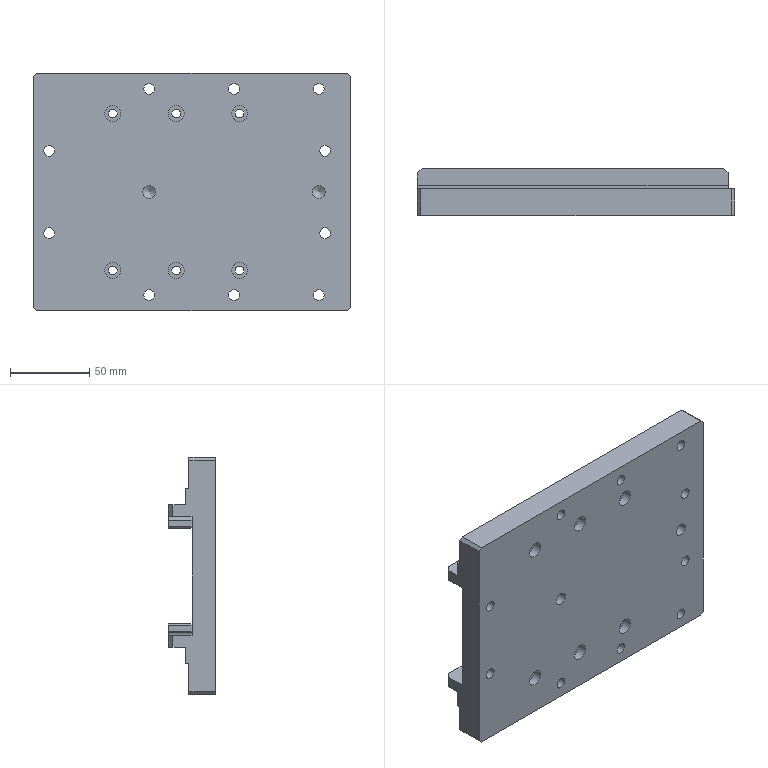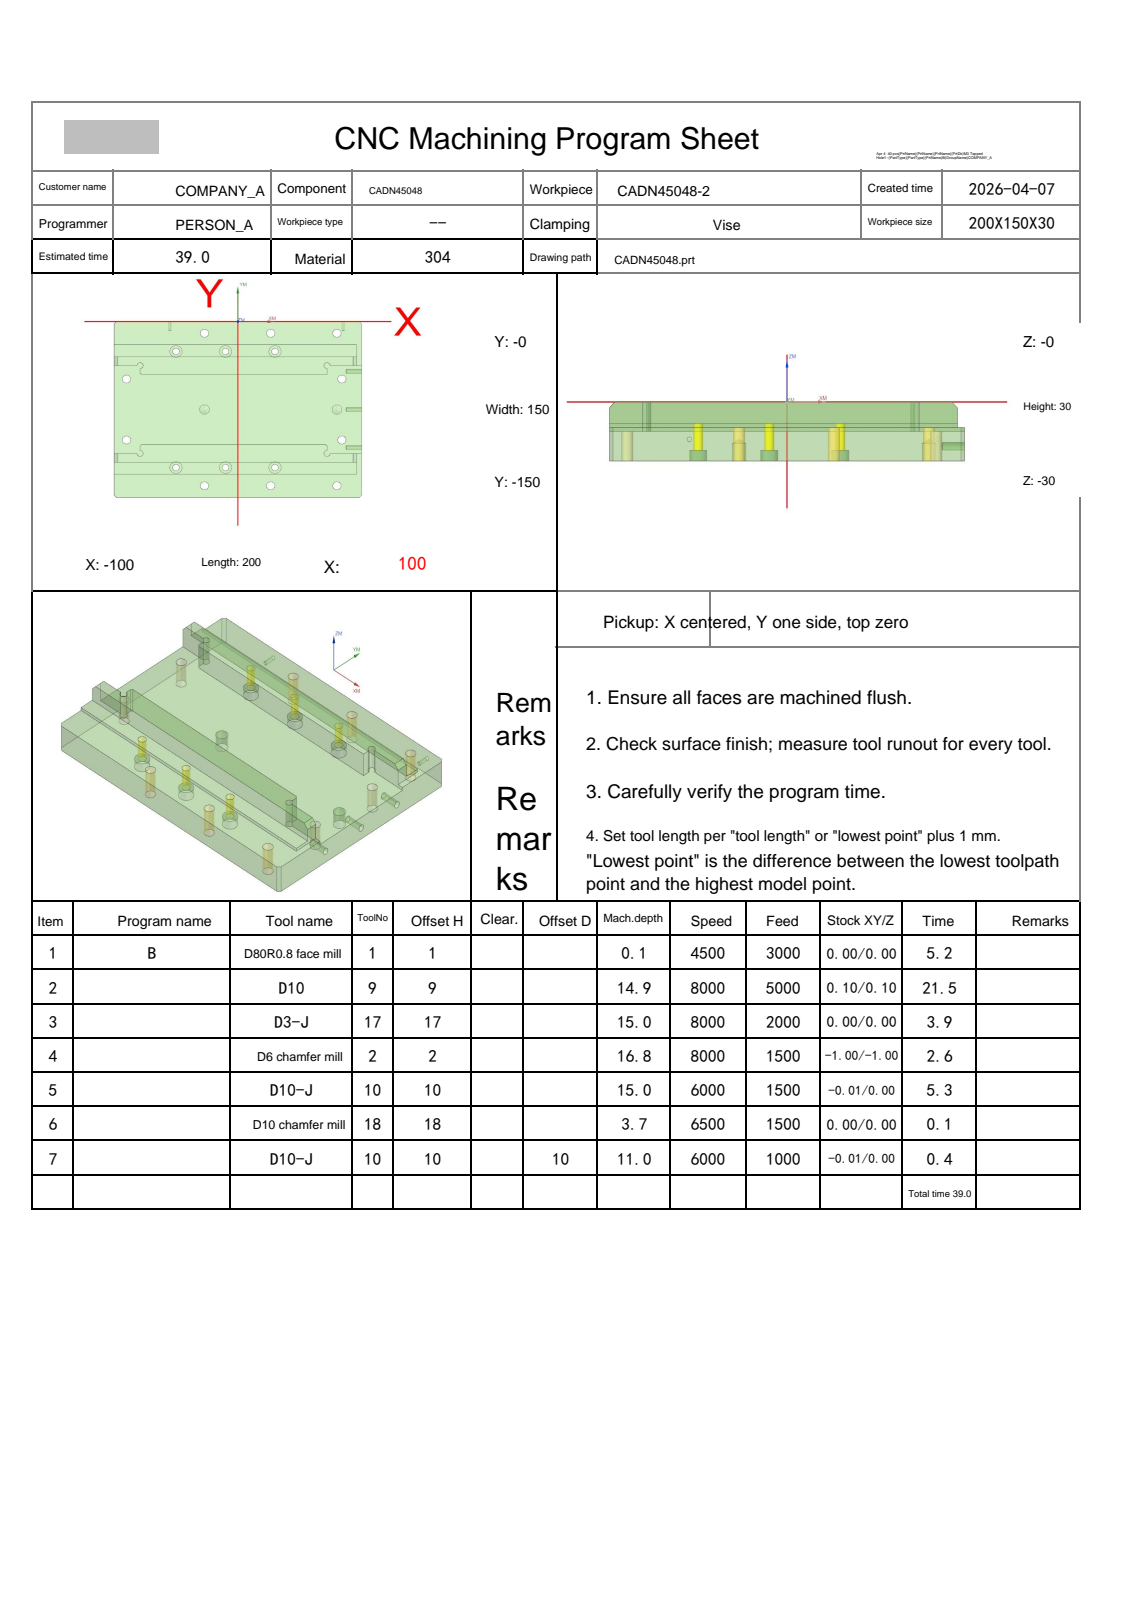NC program | NX | posted by the shop | part box 200 x 30 x 150 mm
Lines 18128 to 19220 of 19220:
N4 T02 M06
(D6 chamfer mill  D=6. R=0. H=02 ce=-1.00 di=-0.80)
G00 G90 G54 X-25. Y-10. M03 S8000
G43 H02 Z20.
M08
Z-13.9
G01 Z-14.4 F600.
X-24.
G03 X-27. Y-7. I-3. J0.0
X-30. Y-10. I0.0 J-3.
X-27. Y-13. I3. J0.0
X-24. Y-10. I0.0 J3.
X-27. Y-7. I-3. J0.0
X-30. Y-10. I0.0 J-3.
G01 X-29.
Z-13.9
G00 Z20.
X28.5
Z-13.9
G01 Z-14.4
X29.5
G03 X26.5 Y-7. I-3. J0.0
X23.5 Y-10. I0.0 J-3.
X26.5 Y-13. I3. J0.0
X29.5 Y-10. I0.0 J3.
X26.5 Y-7. I-3. J0.0
X23.5 Y-10. I0.0 J-3.
G01 X24.5
Z-13.9
G00 Z20.
X82.
Z-13.9
G01 Z-14.4
X83.
G03 X80. Y-7. I-3. J0.0
X77. Y-10. I0.0 J-3.
X80. Y-13. I3. J0.0
X83. Y-10. I0.0 J3.
X80. Y-7. I-3. J0.0
X77. Y-10. I0.0 J-3.
G01 X78.
Z-13.9
G00 Z20.
X83.63 Y-49.152
Z-13.9
G01 Z-14.4
X83.621 Y-49.316
X83.618 Y-49.4
G03 X84. Y-50.4 I1.5 J0.0
X85.4 Y-49. I0.0 J1.4
X84. Y-47.6 I-1.4 J0.0
X82.6 Y-49. I0.0 J-1.4
X84. Y-50.4 I1.4 J0.0
X84.382 Y-49.4 I-1.118 J1.
G01 X84.379 Y-49.316
X84.37 Y-49.152
Z-13.9
G00 Z20.
X83.63 Y-101.152
Z-13.9
G01 Z-14.4
X83.621 Y-101.316
X83.618 Y-101.4
G03 X84. Y-102.4 I1.5 J0.0
X85.4 Y-101. I0.0 J1.4
X84. Y-99.6 I-1.4 J0.0
X82.6 Y-101. I0.0 J-1.4
X84. Y-102.4 I1.4 J0.0
X84.382 Y-101.4 I-1.118 J1.
G01 X84.379 Y-101.316
X84.37 Y-101.152
Z-13.9
G00 Z20.
X82. Y-140.
Z-13.9
G01 Z-14.4
X83.
G03 X80. Y-137. I-3. J0.0
X77. Y-140. I0.0 J-3.
X80. Y-143. I3. J0.0
X83. Y-140. I0.0 J3.
X80. Y-137. I-3. J0.0
X77. Y-140. I0.0 J-3.
G01 X78.
Z-13.9
G00 Z20.
X28.5
Z-13.9
G01 Z-14.4
X29.5
G03 X26.5 Y-137. I-3. J0.0
X23.5 Y-140. I0.0 J-3.
X26.5 Y-143. I3. J0.0
X29.5 Y-140. I0.0 J3.
X26.5 Y-137. I-3. J0.0
X23.5 Y-140. I0.0 J-3.
G01 X24.5
Z-13.9
G00 Z20.
X-25.
Z-13.9
G01 Z-14.4
X-24.
G03 X-27. Y-137. I-3. J0.0
X-30. Y-140. I0.0 J-3.
X-27. Y-143. I3. J0.0
X-24. Y-140. I0.0 J3.
X-27. Y-137. I-3. J0.0
X-30. Y-140. I0.0 J-3.
G01 X-29.
Z-13.9
G00 Z20.
X-90.37 Y-101.152
Z-13.9
G01 Z-14.4
X-90.379 Y-101.316
X-90.382 Y-101.4
G03 X-90. Y-102.4 I1.5 J0.0
X-88.6 Y-101. I0.0 J1.4
X-90. Y-99.6 I-1.4 J0.0
X-91.4 Y-101. I0.0 J-1.4
X-90. Y-102.4 I1.4 J0.0
X-89.618 Y-101.4 I-1.118 J1.
G01 X-89.621 Y-101.316
X-89.63 Y-101.152
Z-13.9
G00 Z20.
X-90.37 Y-49.152
Z-13.9
G01 Z-14.4
X-90.379 Y-49.316
X-90.382 Y-49.4
G03 X-90. Y-50.4 I1.5 J0.0
X-88.6 Y-49. I0.0 J1.4
X-90. Y-47.6 I-1.4 J0.0
X-91.4 Y-49. I0.0 J-1.4
X-90. Y-50.4 I1.4 J0.0
X-89.618 Y-49.4 I-1.118 J1.
G01 X-89.621 Y-49.316
X-89.63 Y-49.152
Z-13.9
G00 Z20.
G00 G90 X-91.5 Y-49.557 M03 S8000
Z20.
Z-16.3
G01 Z-16.8 F600.
Y-50.1
G03 X-90. Y-51.6 I1.5 J0.0
X-87.4 Y-49. I0.0 J2.6
X-90. Y-46.4 I-2.6 J0.0
X-92.6 Y-49. I0.0 J-2.6
X-90. Y-51.6 I2.6 J0.0
X-88.5 Y-50.1 I0.0 J1.5
G01 Y-49.557
Z-16.3
G00 Z20.
X-91.5 Y-101.557
Z-16.3
G01 Z-16.8
Y-102.1
G03 X-90. Y-103.6 I1.5 J0.0
X-87.4 Y-101. I0.0 J2.6
X-90. Y-98.4 I-2.6 J0.0
X-92.6 Y-101. I0.0 J-2.6
X-90. Y-103.6 I2.6 J0.0
X-88.5 Y-102.1 I0.0 J1.5
G01 Y-101.557
Z-16.3
G00 Z20.
X82.5
Z-16.3
G01 Z-16.8
Y-102.1
G03 X84. Y-103.6 I1.5 J0.0
X86.6 Y-101. I0.0 J2.6
X84. Y-98.4 I-2.6 J0.0
X81.4 Y-101. I0.0 J-2.6
X84. Y-103.6 I2.6 J0.0
X85.5 Y-102.1 I0.0 J1.5
G01 Y-101.557
Z-16.3
G00 Z20.
X82.5 Y-49.557
Z-16.3
G01 Z-16.8
Y-50.1
G03 X84. Y-51.6 I1.5 J0.0
X86.6 Y-49. I0.0 J2.6
X84. Y-46.4 I-2.6 J0.0
X81.4 Y-49. I0.0 J-2.6
X84. Y-51.6 I2.6 J0.0
X85.5 Y-50.1 I0.0 J1.5
G01 Y-49.557
Z-16.3
G00 Z20.
G00 G90 X-97.792 Y-111.51 M03 S6500
Z20.
Z.13
G01 Z-1.2 F1500.
G03 X-97.452 Y-111.585 I.601 J1.907
G01 X-97.398 Y-111.595
X-97.349 Y-111.572
X-97.259 Y-111.534
X-97. Y-111.5
X-81.5
G02 X-80.5 Y-112.5 I0.0 J-1.
G03 X-79. Y-114. I1.5 J0.0
X-77.5 Y-112.5 I0.0 J1.5
X-78.377 Y-111.136 I-1.5 J0.0
G01 X-78.681 Y-111.034
X-79. Y-111.
G02 X-80. Y-110. I0.0 J1.
G01 Y-106.
X-79.966 Y-105.741
X-79.866 Y-105.5
X-79.707 Y-105.293
X-78.707 Y-104.293
X-78.5 Y-104.134
X-78.259 Y-104.034
X-78. Y-104.
X71.
X71.259 Y-104.034
X71.5 Y-104.134
X71.707 Y-104.293
X72.707 Y-105.293
X72.866 Y-105.5
X72.966 Y-105.741
X73. Y-106.
Y-110.
G02 X72. Y-111. I-1. J0.0
G03 X70.5 Y-112.5 I0.0 J-1.5
X72. Y-114. I1.5 J0.0
X73.364 Y-113.123 I0.0 J1.5
G01 X73.466 Y-112.819
X73.5 Y-112.5
G02 X74.5 Y-111.5 I1. J0.0
G01 X93.
X93.259 Y-111.534
X93.349 Y-111.572
X93.398 Y-111.595
X93.452 Y-111.585
G03 X93.792 Y-111.51 I-.261 J1.983
G01 Z.13
G00 Z2.55
Y-120.99
Z.13
G01 Z-1.2
G03 X93.452 Y-120.915 I-.601 J-1.907
G01 X93.398 Y-120.905
X93.349 Y-120.928
X93.259 Y-120.966
X93. Y-121.
X-2.
X-97.
X-97.259 Y-120.966
X-97.349 Y-120.928
X-97.398 Y-120.905
X-97.452 Y-120.915
G03 X-97.792 Y-120.99 I.261 J-1.983
G01 Z.13
G00 Z10.
X93.792 Y-38.49
Z.13
G01 Z-1.2
G03 X93.452 Y-38.415 I-.601 J-1.907
G01 X93.398 Y-38.405
X93.349 Y-38.428
X93.259 Y-38.466
X93. Y-38.5
X74.5
G02 X73.5 Y-37.5 I0.0 J1.
G03 X72. Y-36. I-1.5 J0.0
X70.5 Y-37.5 I0.0 J-1.5
X71.377 Y-38.864 I1.5 J0.0
G01 X71.681 Y-38.966
X72. Y-39.
G02 X73. Y-40. I0.0 J-1.
G01 Y-45.
G02 X72. Y-46. I-1. J0.0
G01 X-78.
X-78.259 Y-45.966
X-78.5 Y-45.866
X-78.707 Y-45.707
X-79.707 Y-44.707
X-79.866 Y-44.5
X-79.966 Y-44.259
X-80. Y-44.
Y-40.
G02 X-79. Y-39. I1. J0.0
G03 X-77.5 Y-37.5 I0.0 J1.5
X-79. Y-36. I-1.5 J0.0
X-80.364 Y-36.877 I0.0 J-1.5
G01 X-80.466 Y-37.181
X-80.5 Y-37.5
G02 X-81.5 Y-38.5 I-1. J0.0
G01 X-97.
X-97.259 Y-38.466
X-97.349 Y-38.428
X-97.398 Y-38.405
X-97.452 Y-38.415
G03 X-97.792 Y-38.49 I.261 J-1.983
G01 Z.13
G00 Z2.55
Y-29.01
Z.13
G01 Z-1.2
G03 X-97.452 Y-29.085 I.601 J1.907
G01 X-97.398 Y-29.095
X-97.349 Y-29.072
X-97.259 Y-29.034
X-97. Y-29.
X-2.
X93.
X93.259 Y-29.034
X93.349 Y-29.072
X93.398 Y-29.095
X93.452 Y-29.085
G03 X93.792 Y-29.01 I-.261 J1.983
G01 Z.13
G00 Z10.
X-101.068 Y-26.968
Z-3.305
G01 Z-12.2
X-101.008 Y-26.882
X-101. Y-26.852
Y-19.8
G02 X-100. Y-18.8 I1. J0.0
G01 X96.
G02 X97. Y-19.8 I0.0 J-1.
G01 Y-26.882
X97.005 Y-26.902
X97.045 Y-26.959
Z-3.292
G00 Z10.
X-49.172 Y-26.791
Z-1.81
G01 Z-12.2
G03 X-48.826 Y-26.749 I-.07 J1.999
G01 X-48.772 Y-26.74
X-48.733 Y-26.702
X-48.699 Y-26.671
G03 X-48.25 Y-25.5 I-1.301 J1.171
X-50. Y-23.75 I-1.75 J0.0
X-51.75 Y-25.5 I0.0 J-1.75
X-51.664 Y-26.041 I1.75 J0.0
G01 X-51.516 Y-26.375
X-51.301 Y-26.671
X-51.267 Y-26.702
X-51.232 Y-26.726
X-51.189 Y-26.76
X-51.135 Y-26.763
X-50.94 Y-26.772
X-50.786 Y-26.766
Z-1.835
G00 Z10.
X-9.172 Y-26.791
Z-1.81
G01 Z-12.2
G03 X-8.826 Y-26.749 I-.07 J1.999
G01 X-8.772 Y-26.74
X-8.733 Y-26.702
X-8.699 Y-26.671
G03 X-8.25 Y-25.5 I-1.301 J1.171
X-10. Y-23.75 I-1.75 J0.0
X-11.75 Y-25.5 I0.0 J-1.75
X-11.664 Y-26.041 I1.75 J0.0
G01 X-11.516 Y-26.375
X-11.301 Y-26.671
X-11.267 Y-26.702
X-11.232 Y-26.726
X-11.189 Y-26.76
X-11.135 Y-26.763
X-10.94 Y-26.772
X-10.786 Y-26.766
Z-1.835
G00 Z10.
X30.828 Y-26.791
Z-1.81
G01 Z-12.2
G03 X31.174 Y-26.749 I-.07 J1.999
G01 X31.228 Y-26.74
X31.267 Y-26.702
X31.301 Y-26.671
G03 X31.75 Y-25.5 I-1.301 J1.171
X30.364 Y-23.788 I-1.75 J0.0
G01 X30. Y-23.75
G03 X28.25 Y-25.5 I0.0 J-1.75
X28.484 Y-26.375 I1.75 J0.0
G01 X28.699 Y-26.671
X28.733 Y-26.702
X28.768 Y-26.726
X28.811 Y-26.76
X28.865 Y-26.763
X29.06 Y-26.772
X29.214 Y-26.766
Z-1.835
G00 Z10.
X97.068 Y-123.032
Z-3.305
G01 Z-12.2
X97.008 Y-123.118
X97. Y-123.148
Y-130.2
G02 X96. Y-131.2 I-1. J0.0
G01 X-100.
G02 X-101. Y-130.2 I0.0 J1.
G01 Y-123.118
X-101.005 Y-123.098
X-101.045 Y-123.041
Z-3.292
G00 Z10.
X-50.828 Y-123.209
Z-1.81
G01 Z-12.2
G03 X-51.174 Y-123.251 I.07 J-1.999
G01 X-51.228 Y-123.26
X-51.267 Y-123.298
X-51.301 Y-123.329
G03 X-51.75 Y-124.5 I1.301 J-1.171
X-50. Y-126.25 I1.75 J0.0
X-48.25 Y-124.5 I0.0 J1.75
X-48.336 Y-123.959 I-1.75 J0.0
G01 X-48.484 Y-123.625
X-48.699 Y-123.329
X-48.733 Y-123.298
X-48.768 Y-123.274
X-48.811 Y-123.24
X-48.865 Y-123.237
X-49.06 Y-123.228
X-49.214 Y-123.234
Z-1.835
G00 Z10.
X-10.828 Y-123.209
Z-1.81
G01 Z-12.2
G03 X-11.174 Y-123.251 I.07 J-1.999
G01 X-11.228 Y-123.26
X-11.267 Y-123.298
X-11.301 Y-123.329
G03 X-11.75 Y-124.5 I1.301 J-1.171
X-10. Y-126.25 I1.75 J0.0
X-8.25 Y-124.5 I0.0 J1.75
X-8.336 Y-123.959 I-1.75 J0.0
G01 X-8.484 Y-123.625
X-8.699 Y-123.329
X-8.733 Y-123.298
X-8.768 Y-123.274
X-8.811 Y-123.24
X-8.865 Y-123.237
X-9.06 Y-123.228
X-9.214 Y-123.234
Z-1.835
G00 Z10.
X29.172 Y-123.209
Z-1.81
G01 Z-12.2
G03 X28.826 Y-123.251 I.07 J-1.999
G01 X28.772 Y-123.26
X28.733 Y-123.298
X28.699 Y-123.329
G03 X28.25 Y-124.5 I1.301 J-1.171
X30. Y-126.25 I1.75 J0.0
X31.75 Y-124.5 I0.0 J1.75
X31.664 Y-123.959 I-1.75 J0.0
G01 X31.516 Y-123.625
X31.301 Y-123.329
X31.267 Y-123.298
X31.232 Y-123.274
X31.189 Y-123.24
X31.135 Y-123.237
X30.94 Y-123.228
X30.786 Y-123.234
Z-1.835
G00 Z10.
X99.009 Y-111.432
Z-4.086
G01 Z-14.2
X99.095 Y-111.492
X99.125 Y-111.5
X100.
G02 X101. Y-112.5 I0.0 J-1.
G01 Y-148.
X100.966 Y-148.259
X100.866 Y-148.5
X100.707 Y-148.707
X98.707 Y-150.707
X98.5 Y-150.866
X98.259 Y-150.966
X98. Y-151.
X-98.
X-98.259 Y-150.966
X-98.5 Y-150.866
X-98.707 Y-150.707
X-100.707 Y-148.707
X-100.866 Y-148.5
X-100.966 Y-148.259
X-101. Y-148.
Y-133.294
X-101.008 Y-133.264
X-101.068 Y-133.178
Z-12.669
G00 Z10.
X-26.596 Y-137.792
Z-12.75
G01 Z-14.2
G03 X-26.898 Y-137.618 I-1.147 J-1.638
G01 X-26.946 Y-137.592
X-27. Y-137.6
G03 X-29.4 Y-140. I0.0 J-2.4
X-27. Y-142.4 I2.4 J0.0
X-24.6 Y-140. I0.0 J2.4
X-27. Y-137.6 I-2.4 J0.0
G01 X-27.054 Y-137.592
X-27.102 Y-137.618
G03 X-27.404 Y-137.792 I.845 J-1.813
G01 Z-12.75
G00 Z10.
X26.904
Z-12.75
G01 Z-14.2
G03 X26.602 Y-137.618 I-1.147 J-1.638
G01 X26.554 Y-137.592
X26.5 Y-137.6
G03 X24.1 Y-140. I0.0 J-2.4
X26.5 Y-142.4 I2.4 J0.0
X28.9 Y-140. I0.0 J2.4
X26.5 Y-137.6 I-2.4 J0.0
G01 X26.446 Y-137.592
X26.398 Y-137.618
G03 X26.096 Y-137.792 I.845 J-1.813
G01 Z-12.75
G00 Z10.
X80.404
Z-12.75
G01 Z-14.2
G03 X80.102 Y-137.618 I-1.147 J-1.638
G01 X80.054 Y-137.592
X80. Y-137.6
G03 X77.6 Y-140. I0.0 J-2.4
X80. Y-142.4 I2.4 J0.0
X82.4 Y-140. I0.0 J2.4
X80. Y-137.6 I-2.4 J0.0
G01 X79.946 Y-137.592
X79.898 Y-137.618
G03 X79.596 Y-137.792 I.845 J-1.813
G01 Z-12.75
G00 Z10.
X-101.068 Y-16.822
Z-12.669
G01 Z-14.2
X-101.008 Y-16.736
X-101. Y-16.706
Y-2.
X-100.966 Y-1.741
X-100.866 Y-1.5
X-100.707 Y-1.293
X-98.707 Y.707
X-98.5 Y.866
X-98.259 Y.966
X-98. Y1.
X98.
X98.259 Y.966
X98.5 Y.866
X98.707 Y.707
X100.707 Y-1.293
X100.866 Y-1.5
X100.966 Y-1.741
X101. Y-2.
Y-37.5
G02 X100. Y-38.5 I-1. J0.0
G01 X99.125
X99.095 Y-38.508
X99.009 Y-38.568
Z-4.086
G00 Z10.
X80.404 Y-7.792
Z-12.75
G01 Z-14.2
G03 X80.102 Y-7.618 I-1.147 J-1.638
G01 X80.054 Y-7.592
X80. Y-7.6
G03 X77.6 Y-10. I0.0 J-2.4
X80. Y-12.4 I2.4 J0.0
X82.4 Y-10. I0.0 J2.4
X80. Y-7.6 I-2.4 J0.0
G01 X79.946 Y-7.592
X79.898 Y-7.618
G03 X79.596 Y-7.792 I.845 J-1.813
G01 Z-12.75
G00 Z10.
X26.904
Z-12.75
G01 Z-14.2
G03 X26.602 Y-7.618 I-1.147 J-1.638
G01 X26.554 Y-7.592
X26.5 Y-7.6
G03 X24.1 Y-10. I0.0 J-2.4
X26.5 Y-12.4 I2.4 J0.0
X28.9 Y-10. I0.0 J2.4
X26.5 Y-7.6 I-2.4 J0.0
G01 X26.446 Y-7.592
X26.398 Y-7.618
G03 X26.096 Y-7.792 I.845 J-1.813
G01 Z-12.75
G00 Z10.
X-26.596
Z-12.75
G01 Z-14.2
G03 X-26.898 Y-7.618 I-1.147 J-1.638
G01 X-26.946 Y-7.592
X-27. Y-7.6
G03 X-29.4 Y-10. I0.0 J-2.4
X-27. Y-12.4 I2.4 J0.0
X-24.6 Y-10. I0.0 J2.4
X-27. Y-7.6 I-2.4 J0.0
G01 X-27.054 Y-7.592
X-27.102 Y-7.618
G03 X-27.404 Y-7.792 I.845 J-1.813
G01 Z-12.75
G00 Z10.
X101.091 Y-40.459
Z-14.692
G01 Z-16.2
X101.04 Y-40.508
X101.011 Y-40.573
X100.993 Y-40.59
X101. Y-40.613
Y-109.387
X100.993 Y-109.411
X101.011 Y-109.427
X101.04 Y-109.492
X101.091 Y-109.541
Z-14.692
G00 Z10.
X-101.068 Y-109.466
Z-3.306
G01 Z-16.2
X-101.008 Y-109.381
X-101. Y-109.351
Y-40.619
X-101.005 Y-40.599
X-101.045 Y-40.541
Z-3.292
G00 Z10.
X83.596 Y-51.208
Z-14.75
G01 Z-16.2
G03 X83.898 Y-51.382 I1.147 J1.638
G01 X83.946 Y-51.408
X84. Y-51.4
G03 X86.4 Y-49. I0.0 J2.4
X84. Y-46.6 I-2.4 J0.0
X81.6 Y-49. I0.0 J-2.4
X84. Y-51.4 I2.4 J0.0
G01 X84.054 Y-51.408
X84.102 Y-51.382
G03 X84.404 Y-51.208 I-.845 J1.813
G01 Z-14.75
G00 Z10.
X83.596 Y-103.208
Z-14.75
G01 Z-16.2
G03 X83.898 Y-103.382 I1.147 J1.638
G01 X83.946 Y-103.408
X84. Y-103.4
G03 X86.4 Y-101. I0.0 J2.4
X84. Y-98.6 I-2.4 J0.0
X81.6 Y-101. I0.0 J-2.4
X84. Y-103.4 I2.4 J0.0
G01 X84.054 Y-103.408
X84.102 Y-103.382
G03 X84.404 Y-103.208 I-.845 J1.813
G01 Z-14.75
G00 Z10.
X-90.404
Z-14.75
G01 Z-16.2
G03 X-90.102 Y-103.382 I1.147 J1.638
G01 X-90.054 Y-103.408
X-90. Y-103.4
G03 X-87.6 Y-101. I0.0 J2.4
X-90. Y-98.6 I-2.4 J0.0
X-92.4 Y-101. I0.0 J-2.4
X-90. Y-103.4 I2.4 J0.0
G01 X-89.946 Y-103.408
X-89.898 Y-103.382
G03 X-89.596 Y-103.208 I-.845 J1.813
G01 Z-14.75
G00 Z10.
X-90.404 Y-51.208
Z-14.75
G01 Z-16.2
G03 X-90.102 Y-51.382 I1.147 J1.638
G01 X-90.054 Y-51.408
X-90. Y-51.4
G03 X-87.6 Y-49. I0.0 J2.4
X-90. Y-46.6 I-2.4 J0.0
X-92.4 Y-49. I0.0 J-2.4
X-90. Y-51.4 I2.4 J0.0
G01 X-89.946 Y-51.408
X-89.898 Y-51.382
G03 X-89.596 Y-51.208 I-.845 J1.813
G01 Z-14.75
G00 Z20.
G91 G28 Z0.0
M05
M09
G91 G28 Z0.0
M01
N5 T10 M06
(D10-J  D=10. R=0. H=10 ce=0.40 di=0.00)
G00 G90 G54 X103. Y-133.199 M03 S6000
G43 H10 Z14.5
M08
Z-9.5
G01 Z-11. F1500.
G03 X101. Y-131.2 I-2. J-.001
G01 X-104.
G02 X-105. Y-130.2 I0.0 J1.
G01 Y-129.2
G02 X-104.1 Y-128.3 I.9 J0.0
G01 X100.1
G03 X101. Y-127.4 I0.0 J.9
G01 Y-126.4
G03 X100. Y-125.4 I-1. J0.0
G01 X-105.
G03 X-107. Y-127.4 I0.0 J-2.
G01 Z-9.5
G00 Z-7.
Y-16.801
Z-9.5
G01 Z-11.
G03 X-105. Y-18.8 I2. J.001
G01 X100.001
G02 X101. Y-19.799 I-.001 J-1.
G01 Y-19.8
Y-20.701
G02 X100.001 Y-21.7 I-1. J.001
G01 X-104.1
G03 X-105. Y-22.6 I0.0 J-.9
G01 Y-23.6
G03 X-104. Y-24.6 I1. J0.0
G01 X101.
G03 X103. Y-22.6 I0.0 J2.
G01 Z-9.5
G00 Z14.5
G00 G90 X-105.838 Y2.062 M03 S6000
Z14.5
Z-11.5
G01 Z-13. F1500.
G03 X-104.071 Y1. I1.766 J.938
G01 X103.658
G02 X104.363 Y.708 I-.001 J-1.
G01 X104.707 Y.364
G02 X105. Y-.343 I-.707 J-.707
G01 Y-1.851
G02 X104.001 Y-2.85 I-1. J.001
G01 X-104.1
G03 X-105. Y-3.75 I0.0 J-.9
G01 Y-5.7
G03 X-104. Y-6.7 I1. J0.0
G01 X104.1
G02 X105. Y-7.6 I0.0 J-.9
G01 Y-9.55
G02 X104. Y-10.55 I-1. J0.0
G01 X-104.1
G03 X-105. Y-11.45 I0.0 J-.9
G01 Y-13.4
G03 X-104. Y-14.4 I1. J0.0
G01 X105.
G03 X107. Y-12.401 I0.0 J2.
G01 Z-11.5
G00 Z-9.
X105.838 Y-152.062
Z-11.5
G01 Z-13.
G03 X104.071 Y-151. I-1.766 J-.938
G01 X-103.658
G02 X-104.363 Y-150.708 I.001 J1.
G01 X-104.707 Y-150.364
G02 X-105. Y-149.657 I.707 J.707
G01 Y-148.149
G02 X-104.001 Y-147.15 I1. J-.001
G01 X104.1
G03 X105. Y-146.25 I0.0 J.9
G01 Y-144.3
G03 X104. Y-143.3 I-1. J0.0
G01 X-104.1
G02 X-105. Y-142.4 I0.0 J.9
G01 Y-140.45
G02 X-104. Y-139.45 I1. J0.0
G01 X104.1
G03 X105. Y-138.55 I0.0 J.9
G01 Y-136.6
G03 X104. Y-135.6 I-1. J0.0
G01 X-105.
G03 X-107. Y-137.6 I0.0 J-2.
G01 Z-11.5
G00 Z14.5
G00 G90 X107. Y-73.479 M03 S6000
Z14.5
Z-13.5
G01 Z-15. F1500.
X103.
G03 X101. Y-75.479 I0.0 J-2.
G01 Y-106.104
G02 X100.004 Y-107.1 I-1. J.004
G01 X78.396
G02 X77.4 Y-106.104 I.004 J1.
G01 Y-103.763
X73.237 Y-99.6
X-80.237
X-84.4 Y-103.763
Y-106.104
G02 X-85.396 Y-107.1 I-1. J.004
G01 X-100.004
G02 X-101. Y-106.104 I.004 J1.
G01 Y-43.896
G02 X-100.004 Y-42.9 I1. J-.004
G01 X-85.396
G02 X-84.4 Y-43.896 I-.004 J-1.
G01 Y-46.237
X-80.237 Y-50.4
X77.4
Y-43.896
G02 X78.396 Y-42.9 I1. J-.004
G01 X100.004
G02 X101. Y-43.896 I-.004 J-1.
G01 Y-77.565
G02 X100.707 Y-78.271 I-1. J.001
G01 X96.293 Y-82.686
G03 X96. Y-83.392 I.707 J-.707
G01 Y-101.104
G02 X95.004 Y-102.1 I-1. J.004
G01 X82.772
G02 X81.882 Y-101.547 I.004 J1.
G03 X80.936 Y-100.228 I-4.482 J-2.216
G01 X76.772 Y-96.064
G03 X73.237 Y-94.6 I-3.536 J-3.536
G01 X-80.237
G03 X-83.772 Y-96.064 I0.0 J-5.
G01 X-87.936 Y-100.228
G03 X-88.882 Y-101.547 I3.536 J-3.536
G02 X-89.772 Y-102.1 I-.894 J.447
G01 X-95.004
G02 X-96. Y-101.104 I.004 J1.
G01 Y-48.896
G02 X-95.004 Y-47.9 I1. J-.004
G01 X-89.772
G02 X-88.882 Y-48.453 I-.004 J-1.
G03 X-87.936 Y-49.772 I4.482 J2.216
G01 X-83.772 Y-53.936
G03 X-80.237 Y-55.4 I3.536 J3.536
G01 X77.4
G03 X82.4 Y-50.4 I0.0 J5.
G01 Y-48.896
G02 X83.396 Y-47.9 I1. J-.004
G01 X95.004
G02 X96. Y-48.896 I-.004 J-1.
G01 Y-77.565
G02 X95.707 Y-78.271 I-1. J0.0
G01 X91.293 Y-82.686
G03 X91. Y-83.393 I.707 J-.707
G01 Y-96.105
G02 X90.005 Y-97.1 I-1. J.005
G01 X85.287
G02 X84.577 Y-96.8 I.005 J1.
G01 X84.471 Y-96.692
X80.308 Y-92.529
G03 X73.237 Y-89.6 I-7.071 J-7.071
G01 X-80.237
G03 X-87.308 Y-92.529 I0.0 J-10.
G01 X-89.296 Y-94.517
G02 X-90. Y-94.807 I-.704 J.71
X-91. Y-93.812 I0.0 J1.
G01 Y-56.188
G02 X-90. Y-55.193 I1. J-.005
X-89.296 Y-55.483 I0.0 J-1.
G01 X-87.308 Y-57.471
G03 X-80.237 Y-60.4 I7.071 J7.071
G01 X77.4
G03 X86.882 Y-53.578 I0.0 J10.
G02 X87.824 Y-52.9 I.947 J-.322
G01 X90.005
G02 X91. Y-53.895 I-.005 J-1.
G01 Y-77.565
G02 X90.707 Y-78.271 I-1. J0.0
G01 X86.293 Y-82.686
G03 X86. Y-83.393 I.707 J-.707
G01 Y-88.741
G02 X85. Y-89.736 I-1. J.005
X84.297 Y-89.447 I0.0 J1.
G01 X83.843 Y-88.993
G03 X73.237 Y-84.6 I-10.607 J-10.607
G01 X-80.237
G03 X-84.707 Y-85.282 I0.0 J-15.
G02 X-85. Y-85.325 I-.293 J.956
X-86. Y-84.331 I0.0 J1.
G01 Y-65.669
G02 X-85. Y-64.675 I1. J-.005
X-84.707 Y-64.718 I0.0 J-1.
G03 X-80.237 Y-65.4 I4.47 J14.318
G01 X77.4
G03 X84.53 Y-63.597 I0.0 J15.
G02 X85. Y-63.48 I.471 J-.882
X86. Y-64.474 I0.0 J-1.
G01 Y-77.284
G02 X85.349 Y-78.221 I-1. J0.0
G01 X81.439 Y-79.678
G03 X80.894 Y-80.167 I.349 J-.937
G02 X80. Y-80.719 I-.894 J.448
X79.683 Y-80.667 I0.0 J1.
G03 X73.237 Y-79.6 I-6.446 J-18.933
G01 X-80.006
G02 X-81. Y-78.606 I.006 J1.
G01 Y-71.394
G02 X-80.006 Y-70.4 I1. J-.006
G01 X77.4
G03 X79.882 Y-70.245 I0.0 J20.
G01 X80. Y-70.238
G02 X81. Y-71.233 I0.0 J-1.
G01 Y-79.724
X80.992 Y-79.845
G02 X80.43 Y-80.622 I-.992 J.126
G03 X79.291 Y-82.427 I.861 J-1.805
X79.486 Y-83.288 I2. J0.0
G01 Z-13.5
G00 Z14.5
G00 G90 X102.989 Y-105.49 M03 S6000
Z14.5
Z-12.
G01 Z-13. F1000.
G41 D10
X102.79 Y-105.51
G03 X100.99 Y-107.5 I.2 J-1.99
G01 Y-135.19
X-105.
G03 X-106.99 Y-136.99 I0.0 J-2.
G01 G40 X-107.01 Y-137.189
Z-12.
G00 Z3.
Y-12.811
Z-12.
G01 Z-13.
G41 D10
X-106.99 Y-13.01
G03 X-105. Y-14.81 I1.99 J.2
G01 X100.99
Y-42.5
G03 X102.79 Y-44.49 I2. J0.0
G01 G40 X102.989 Y-44.51
Z-12.
G00 Z14.5
G00 G90 X-107.01 Y-105.511 M03 S6000
Z14.5
Z-6.5
G01 Z-7.5 F1000.
G41 D10
X-106.99 Y-105.71
G03 X-105. Y-107.51 I1.99 J.2
G01 X-83.99
Y-103.933
X-80.067 Y-100.01
X73.067
X76.99 Y-103.933
Y-107.51
X105.
G03 X107. Y-105.51 I0.0 J2.
G01 G40 Y-105.31
Z-6.5
G00 Y-44.69
G01 Z-7.5
G41 D10
Y-44.49
G03 X105. Y-42.49 I-2. J0.0
G01 X76.99
Y-49.99
X-80.067
X-83.99 Y-46.067
Y-42.49
X-105.
G03 X-106.99 Y-44.29 I0.0 J-2.
G01 G40 X-107.01 Y-44.489
Z-6.5
G00 Y-105.511
Z-14.
G01 Z-15.
G41 D10
X-106.99 Y-105.71
G03 X-105. Y-107.51 I1.99 J.2
G01 X-83.99
Y-103.933
X-80.067 Y-100.01
X73.067
X76.99 Y-103.933
Y-107.51
X105.
G03 X106.99 Y-105.71 I0.0 J2.
G01 G40 X107.01 Y-105.511
Z-14.
G00 Y-44.489
G01 Z-15.
G41 D10
X106.99 Y-44.29
G03 X105. Y-42.49 I-1.99 J-.2
G01 X76.99
Y-49.99
X-80.067
X-83.99 Y-46.067
Y-42.49
X-105.
G03 X-106.99 Y-44.29 I0.0 J-2.
G01 G40 X-107.01 Y-44.489
Z-14.
G00 Z14.5
G91 G28 Z0.0
M05
M09
G91 G28 Z0.0
M01
N6 T18 M06
(D10 chamfer mill  D=10. R=0. H=18 ce=0.00 di=0.00)
G00 G90 G54 X-101.028 Y-43.2 M03 S6500
G43 H18 Z20.
M08
Z-2.2
G01 Z-3.7 F1500.
G03 X-100.7 Y-42.103 I-1.672 J1.097
G01 Y-25.397
G03 X-101.028 Y-24.3 I-2. J0.0
G01 Z-2.2
G00 Z20.
Y-125.7
Z-2.2
G01 Z-3.7
G03 X-100.7 Y-124.603 I-1.672 J1.097
G01 Y-107.897
G03 X-101.028 Y-106.8 I-2. J0.0
G01 Z-2.2
G00 Z20.
X97.028
Z-2.2
G01 Z-3.7
G03 X96.7 Y-107.897 I1.672 J-1.097
G01 Y-124.603
G03 X97.028 Y-125.7 I2. J0.0
G01 Z-2.2
G00 Z20.
Y-24.3
Z-2.2
G01 Z-3.7
G03 X96.7 Y-25.397 I1.672 J-1.097
G01 Y-42.103
G03 X97.028 Y-43.2 I2. J0.0
G01 Z-2.2
G00 Z20.
G91 G28 Z0.0
M05
M09
G91 G28 Z0.0
M01
N7 T10 M06
(D10-J  D=10. R=0. H=10 ce=-0.01 di=0.00)
G00 G90 G54 X103.01 Y-126.989 M03 S6000
G43 H10 Z14.5
M08
Z-10.
G01 Z-11. F1000.
G41 D10
X102.99 Y-126.79
G03 X101. Y-124.99 I-1.99 J-.2
G01 X-105.
G03 X-106.99 Y-126.79 I0.0 J-2.
G01 G40 X-107.01 Y-126.989
Z-10.
G00 Z3.
Y-23.011
Z-10.
G01 Z-11.
G41 D10
X-106.99 Y-23.21
G03 X-105. Y-25.01 I1.99 J.2
G01 X101.
G03 X102.99 Y-23.21 I0.0 J2.
G01 G40 X103.01 Y-23.011
Z-10.
G00 Z14.5
M05
M09
G91 G28 Z0.0
G91 G28 Y0.0
M30
%